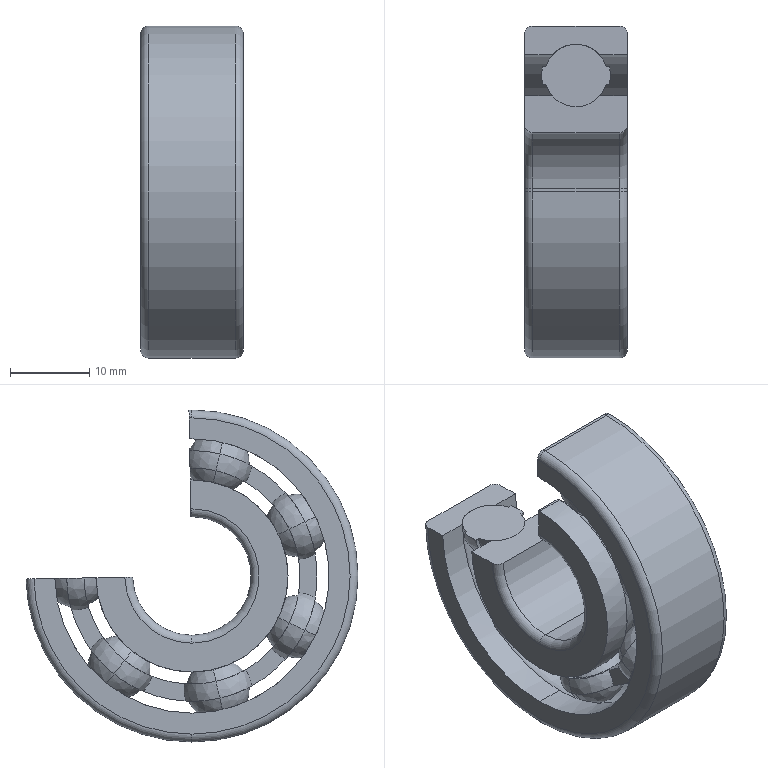Part | STEP file | Bearing 6302 | 1 solid | 122 faces | box 13 x 41.997 x 42 mm | volume 7881 mm3 | sphere 44 | torus 33 | cylinder 26 | plane 19 | commonest cylinder face diameters 24.3 x6 34.7 x6 27.317 x4 31.683 x4 15 x3 42 x3